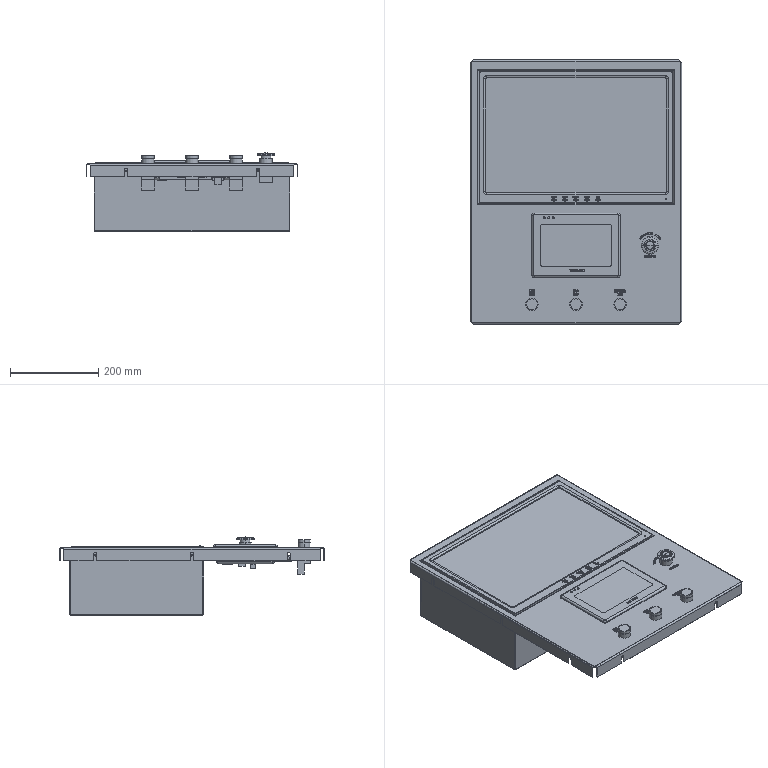Part | SolidWorks | 19 solids | 2648 faces | box 480 x 600 x 177.209 mm | volume 8711349 mm3 | plane 1622 | spline 597 | cylinder 321 | torus 62 | cone 36 | sphere 10 | commonest cylinder face diameters 4 x68 8 x46 1 x37 2 x33 3.3 x16 28.2 x14